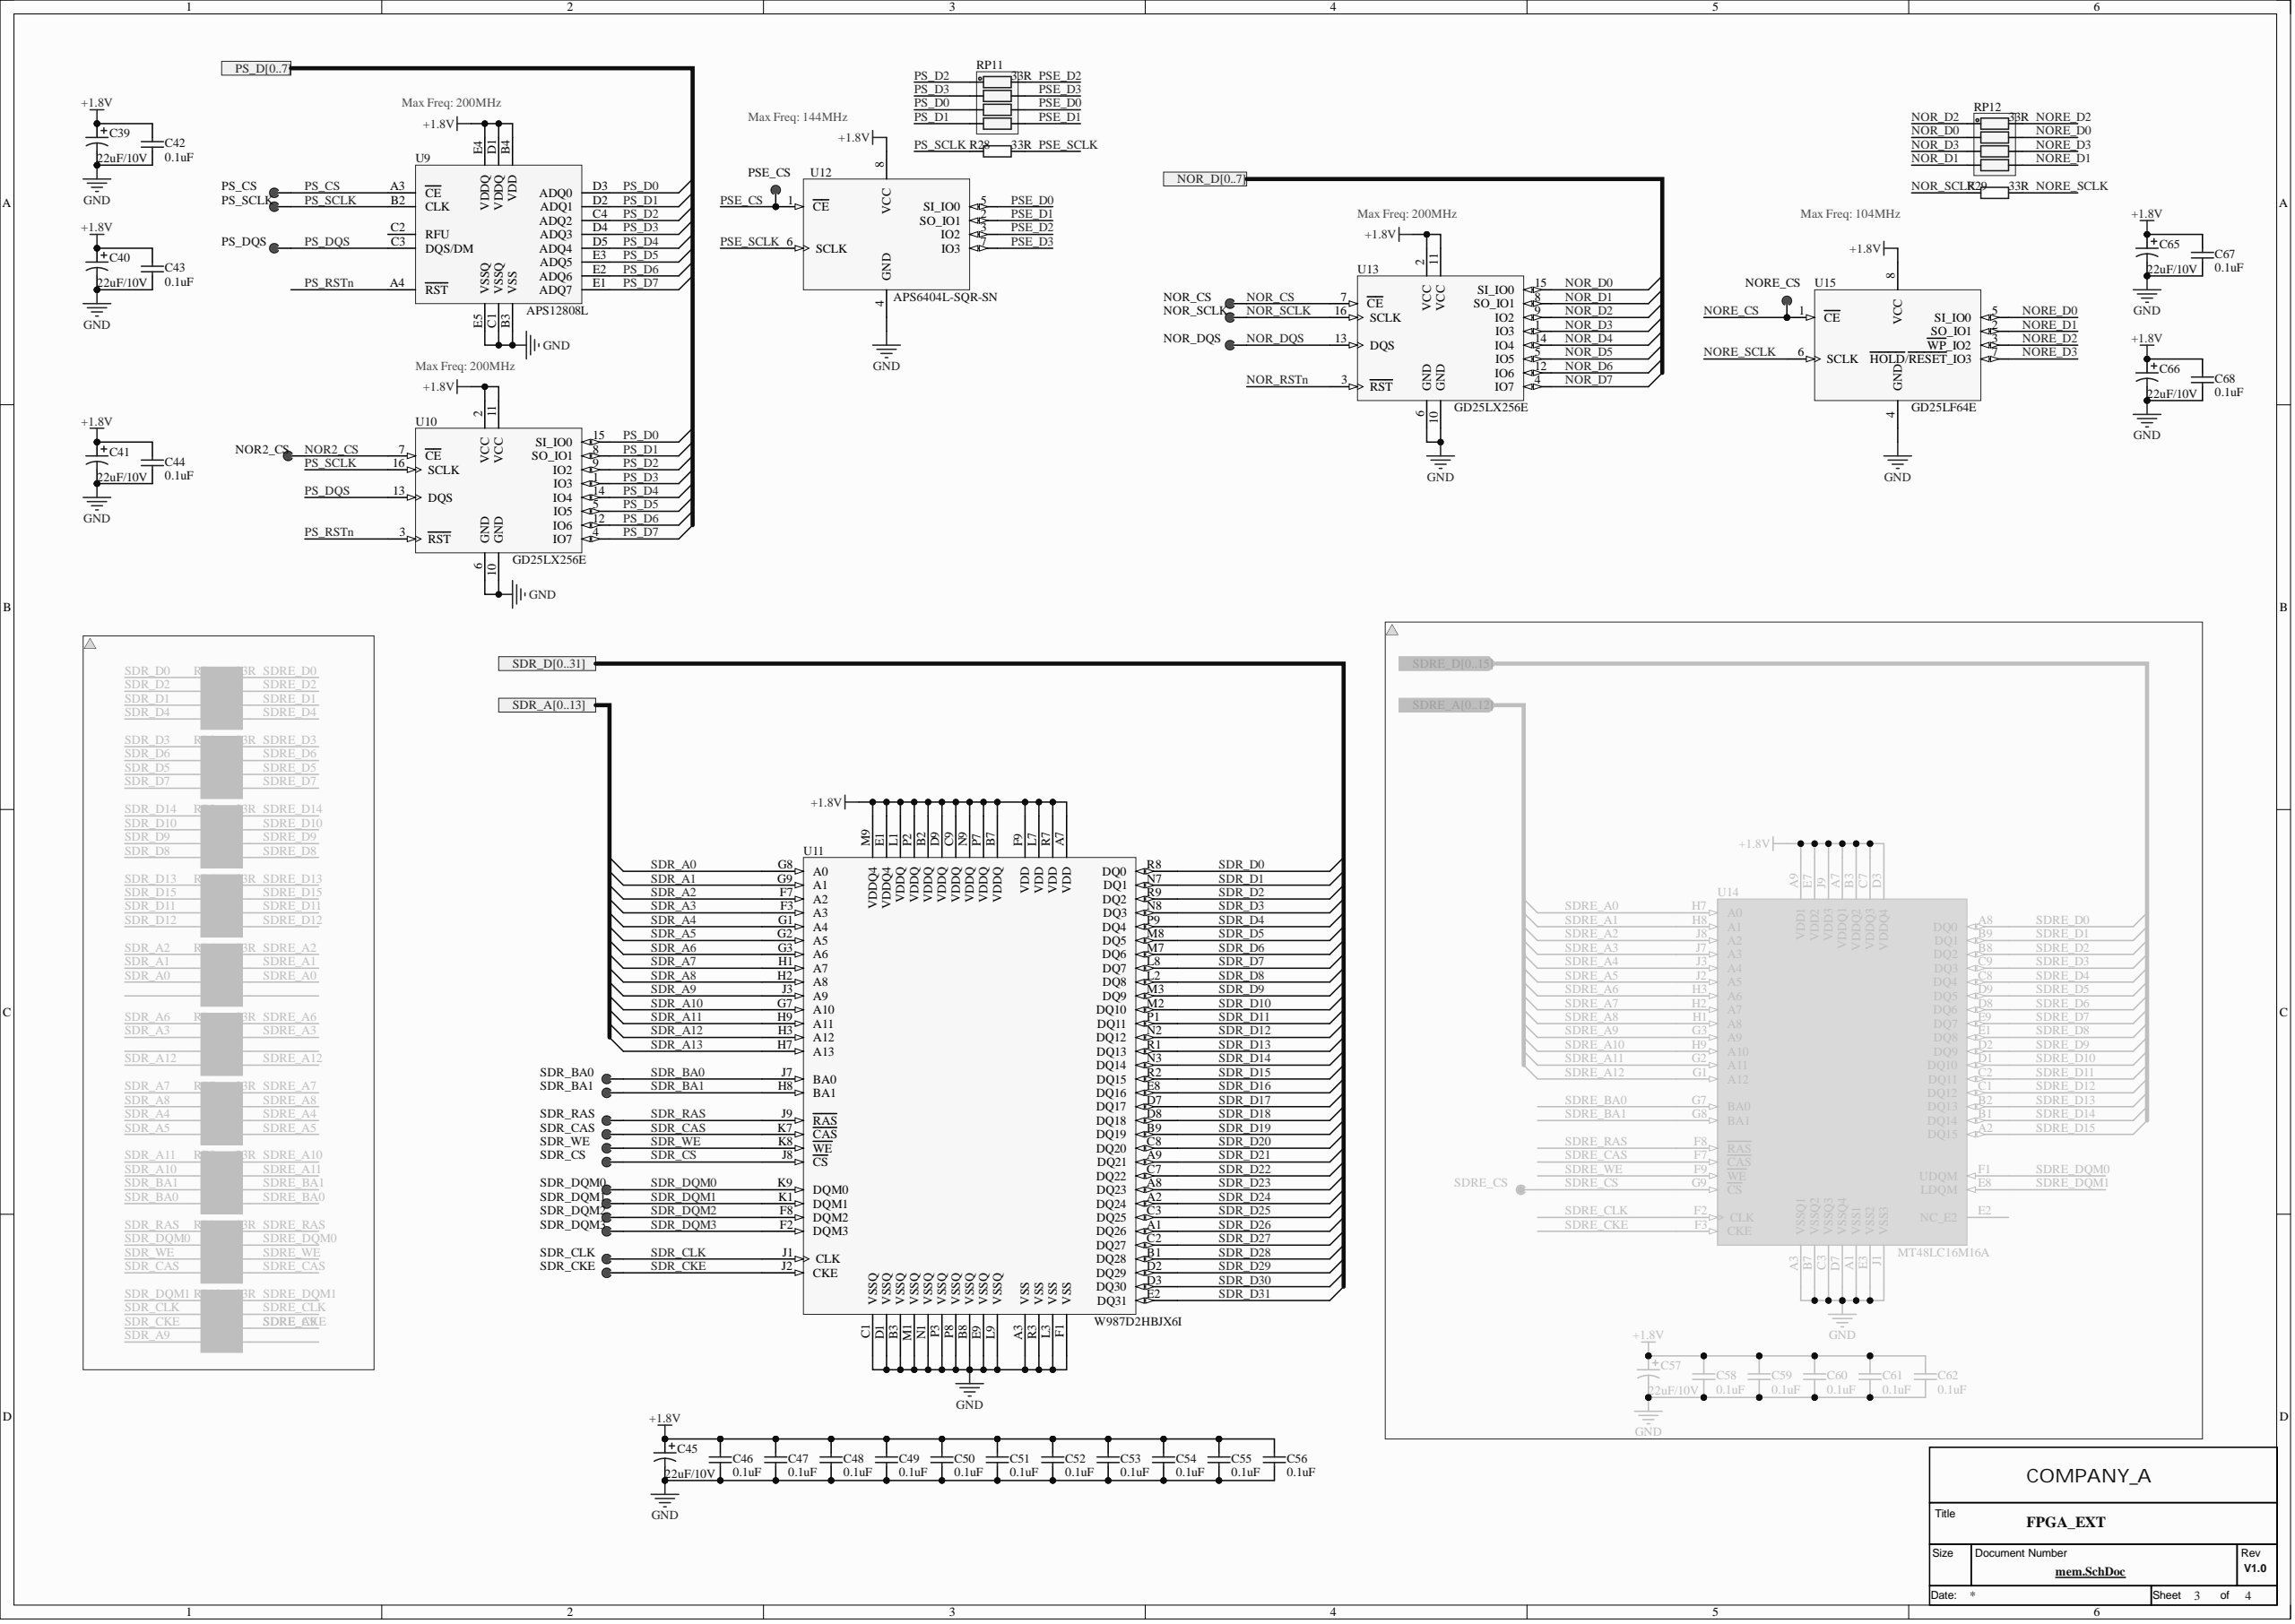Circuit board | Altium Designer | 234 parts | 308 nets | one sheet of the schematic
Parts on this sheet (reference | value | footprint):
C4 | 22uF/10V | 0603C_N
C39 | 22uF/10V | 0603C_N
C40 | 22uF/10V | 0603C_N
C41 | 22uF/10V | 0603C_N
C42 | 0.1uF | 0603C_N
C43 | 0.1uF | 0603C_N
C44 | 0.1uF | 0603C_N
C45 | 22uF/10V | 0603C_N
C46 | 0.1uF | 0603C_N
C47 | 0.1uF | 0603C_N
C48 | 0.1uF | 0603C_N
C49 | 0.1uF | 0603C_N
C50 | 0.1uF | 0603C_N
C51 | 0.1uF | 0603C_N
C52 | 0.1uF | 0603C_N
C53 | 0.1uF | 0603C_N
C54 | 0.1uF | 0603C_N
C55 | 0.1uF | 0603C_N
C56 | 0.1uF | 0603C_N
C65 | 22uF/10V | 0603C_N
C66 | 22uF/10V | 0603C_N
C67 | 0.1uF | 0603C_N
C68 | 0.1uF | 0603C_N
J1 | ASP-184330-01 | ASP-184330-01_Bottom
J2 | FPC0.5-50P | FPC0.5-50P
J3 | FPC0.5-40P | FPC0.5-40P
R28 | 33R | 0603R_N
R29 | 33R | 0603R_N
RP11 | 33R | 0402RP-4P
RP12 | 33R | 0402RP-4P
U9 | APS12808L | PBGA24 6X8
U10 | GD25LX256E | SOIC16
U11 | W987D2HBJX6I | VFBGA90_8X13
U12 | APS6404L-SQR-SN | SOP8
U13 | GD25LX256E | SOIC16
U15 | GD25LF64E | SOIC8
Nets of these parts (net: part-pin ...):
SDR_WE: U11-K8
SDR_RAS: U11-J9
SDR_DQM3: U11-F2
SDR_DQM2: U11-F8
SDR_DQM1: U11-K1
SDR_DQM0: U11-K9
SDR_D31: U11-E2
SDR_D30: U11-D3
SDR_D29: U11-D2
SDR_D28: U11-B1
SDR_D27: U11-C2
SDR_D26: U11-A1
SDR_D25: U11-C3
SDR_D24: U11-A2
SDR_D23: U11-A8
SDR_D22: U11-C7
SDR_D21: U11-A9
SDR_D20: U11-C8
SDR_D19: U11-B9
SDR_D18: U11-D8
SDR_D17: U11-D7
SDR_D16: U11-E8
SDR_D15: U11-R2
SDR_D14: U11-N3
SDR_D13: U11-R1
SDR_D12: U11-N2
SDR_D11: U11-P1
SDR_D10: U11-M2
SDR_D9: U11-M3
SDR_D8: U11-L2
SDR_D7: U11-L8
SDR_D6: U11-M7
SDR_D5: U11-M8
SDR_D4: U11-P9
SDR_D3: U11-N8
SDR_D2: U11-R9
SDR_D1: U11-N7
SDR_D0: U11-R8
SDR_CS: U11-J8
SDR_CLK: U11-J1
SDR_CKE: U11-J2
SDR_CAS: U11-K7
SDR_BA1: U11-H8
SDR_BA0: U11-J7
SDR_A13: J1-G7 U11-H7
SDR_A12: U11-H3
SDR_A11: U11-H9
SDR_A10: U11-G7
SDR_A9: U11-J3
SDR_A8: U11-H2
SDR_A7: U11-H1
SDR_A6: U11-G3
SDR_A5: U11-G2
SDR_A4: U11-G1
SDR_A3: U11-F3
SDR_A2: U11-F7
SDR_A1: U11-G9
SDR_A0: U11-G8
PSE_SCLK: R28-1 U12-6
PSE_D3: RP11-7 U12-7
PSE_D2: RP11-8 U12-3
PSE_D1: RP11-5 U12-2
PSE_D0: RP11-6 U12-5
PSE_CS: U12-1 J1-M2
PS_SCLK: R28-2 U9-B2 U10-16
PS_RSTn: U9-A4 U10-3
PS_DQS: U9-C3 U10-13
PS_D7: U9-E1 U10-4
PS_D6: U9-E2 U10-12
PS_D5: U9-E3 U10-5
PS_D4: U9-D5 U10-14
PS_D3: RP11-2 U9-D4 U10-1 J1-L9
PS_D2: RP11-1 U9-C4 U10-9 J1-L8
PS_D1: RP11-4 U9-D2 U10-8 J1-M7
PS_D0: RP11-3 U9-D3 U10-15
PS_CS: U9-A3
NORE_SCLK: R29-1 U15-6
NORE_D3: RP12-6 U15-7
NORE_D2: RP12-8 U15-3
NORE_D1: RP12-5 U15-2
NORE_D0: RP12-7 U15-5
NORE_CS: U15-1
NOR_SCLK: R29-2 U13-16 J1-J7
NOR_DQS: U13-13
NOR_D7: U13-4
NOR_D6: U13-12
NOR_D5: U13-5
NOR_D4: U13-14
NOR_D3: RP12-3 U13-1
NOR_D2: RP12-1 U13-9 J1-J9
NOR_D1: RP12-4 U13-8 J1-K8
NOR_D0: RP12-2 U13-15 J1-K7
NOR_CS: U13-7
NOR2_CS: U10-7 J1-M3
LCD_DVDD: C4-1 J2-7 J3-4
GND: C4-2 C39-2 C40-2 C41-2 C42-1 C43-1 C44-1 C45-2 C46-1 C47-1 C48-1 C49-1 C50-1 C51-1 C52-1 C53-1 C54-1 C55-1 C56-1 C65-2 C66-2 C67-1 C68-1 U9-B3 U9-C1 U9-E5 U10-6 U10-10 U12-4 U13-6 U13-10 U15-4 J1-A1 J1-A4 J1-A5 J1-A8 J1-A9 J1-A12 J1-A13 J1-B2 J1-B3 J1-B7 J1-C1 J1-C4 J1-C8 J1-C9 J1-C40 J1-D2 J1-D3 J1-D7 J1-E1 J1-E4 J1-E5 J1-E8 J1-F2 J1-F3 J1-F9 J1-G1 J1-G8 J1-H3 J1-H9 J1-J1 J1-J8 J1-K9 J1-L2 J1-L3 J1-L7 J1-M1 J1-M8 J1-M9 J2-5 J3-3 U11-A3 U11-B3 U11-B8 U11-C1 U11-D1 U11-E9 U11-F1 U11-L3 U11-L9 U11-M1 U11-N1 U11-P3 U11-P8 U11-R3
+1.8V: C39-1 C40-1 C41-1 C42-2 C43-2 C44-2 C45-1 C46-2 C47-2 C48-2 C49-2 C50-2 C51-2 C52-2 C53-2 C54-2 C55-2 C56-2 C65-1 C66-1 C67-2 C68-2 U9-B4 U9-D1 U9-E4 U10-2 U10-11 U12-8 U13-2 U13-11 U15-8 U11-A7 U11-B2 U11-B7 U11-C9 U11-D9 U11-E1 U11-F9 U11-L1 U11-L7 U11-M9 U11-N9 U11-P2 U11-P7 U11-R7